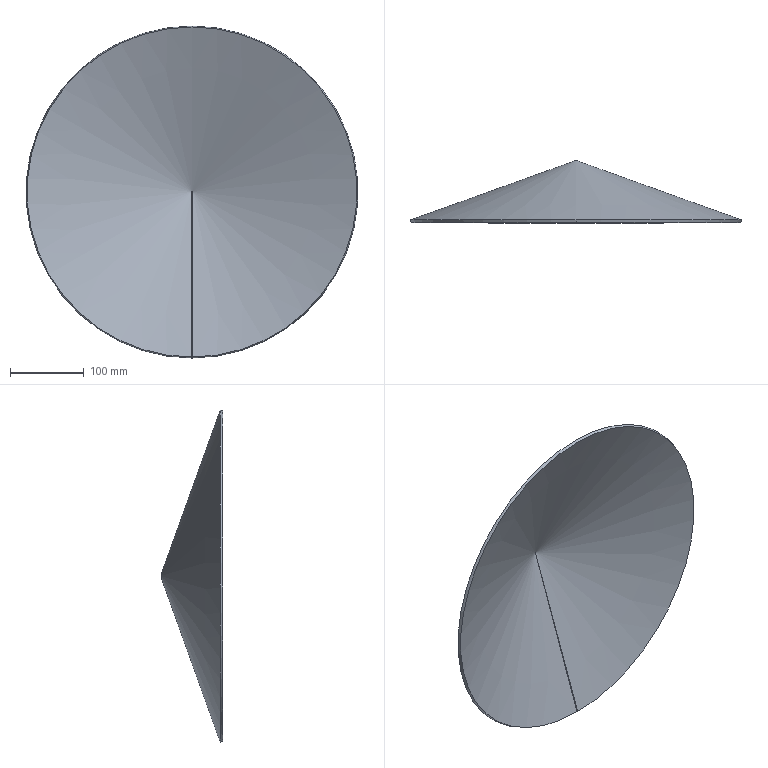Part | SolidWorks | features FlatPattern 1, LoftedBend 1, SheetMetal 1 | 1 solid | 8 faces | box 450 x 83.765 x 449.999 mm | volume 671050 mm3 | cone 6 | plane 2
STEP:
#1=CARTESIAN_POINT('',(0.,-3.765,223.649));
#2=VERTEX_POINT('',#1);
#3=CARTESIAN_POINT('',(-0.7807,-3.765,-223.648));
#4=VERTEX_POINT('',#3);
#5=CARTESIAN_POINT('',(0.,-3.765,0.));
#6=DIRECTION('',(0.,-1.,0.));
#7=DIRECTION('',(0.,0.,-1.));
#8=AXIS2_PLACEMENT_3D('',#5,#6,#7);
#9=CIRCLE('',#8,223.649);
#10=EDGE_CURVE('',#2,#4,#9,.T.);
#11=ORIENTED_EDGE('',*,*,#10,.F.);
#12=CARTESIAN_POINT('',(0.,0.,225.));
#13=VERTEX_POINT('',#12);
#14=CARTESIAN_POINT('',(0.,0.,225.));
#15=DIRECTION('',(0.,0.9413,0.3377));
#16=VECTOR('',#15,1000.);
#17=LINE('',#14,#16);
#18=EDGE_CURVE('',#2,#13,#17,.T.);
#19=ORIENTED_EDGE('',*,*,#18,.T.);
#20=CARTESIAN_POINT('',(-0.7854,0.,-224.999));
#21=VERTEX_POINT('',#20);
#22=CARTESIAN_POINT('',(0.,0.,0.));
#23=DIRECTION('',(0.,-1.,0.));
#24=DIRECTION('',(0.,0.,-1.));
#25=AXIS2_PLACEMENT_3D('',#22,#23,#24);
#26=CIRCLE('',#25,225.);
#27=EDGE_CURVE('',#13,#21,#26,.T.);
#28=ORIENTED_EDGE('',*,*,#27,.T.);
#29=CARTESIAN_POINT('',(-0.7854,0.,-224.999));
#30=DIRECTION('',(-0.001179,0.9413,-0.3377));
#31=VECTOR('',#30,1000.);
#32=LINE('',#29,#31);
#33=EDGE_CURVE('',#4,#21,#32,.T.);
#34=ORIENTED_EDGE('',*,*,#33,.F.);
#35=EDGE_LOOP('',(#11,#19,#28,#34));
#36=FACE_OUTER_BOUND('',#35,.T.);
#37=CARTESIAN_POINT('',(0.,0.,0.));
#38=DIRECTION('',(0.,1.,0.));
#39=DIRECTION('',(0.,0.,1.));
#40=AXIS2_PLACEMENT_3D('',#37,#38,#39);
#41=CONICAL_SURFACE('',#40,225.,0.3444);
#42=ADVANCED_FACE('',(#36),#41,.T.);
#43=CARTESIAN_POINT('',(0.002267,76.235,-0.6493));
#44=VERTEX_POINT('',#43);
#45=CARTESIAN_POINT('',(0.,76.235,0.6493));
#46=VERTEX_POINT('',#45);
#47=CARTESIAN_POINT('',(0.,76.235,0.));
#48=DIRECTION('',(0.,-1.,0.));
#49=DIRECTION('',(0.,0.,-1.));
#50=AXIS2_PLACEMENT_3D('',#47,#48,#49);
#51=CIRCLE('',#50,0.6493);
#52=EDGE_CURVE('',#44,#46,#51,.T.);
#53=ORIENTED_EDGE('',*,*,#52,.T.);
#54=CARTESIAN_POINT('',(0.,80.,2.));
#55=VERTEX_POINT('',#54);
#56=CARTESIAN_POINT('',(0.,80.,2.));
#57=DIRECTION('',(0.,0.9413,0.3377));
#58=VECTOR('',#57,1000.);
#59=LINE('',#56,#58);
#60=EDGE_CURVE('',#46,#55,#59,.T.);
#61=ORIENTED_EDGE('',*,*,#60,.T.);
#62=CARTESIAN_POINT('',(0.006981,80.,-2.));
#63=VERTEX_POINT('',#62);
#64=CARTESIAN_POINT('',(0.,80.,0.));
#65=DIRECTION('',(0.,-1.,0.));
#66=DIRECTION('',(0.,0.,-1.));
#67=AXIS2_PLACEMENT_3D('',#64,#65,#66);
#68=CIRCLE('',#67,2.);
#69=EDGE_CURVE('',#63,#55,#68,.T.);
#70=ORIENTED_EDGE('',*,*,#69,.F.);
#71=CARTESIAN_POINT('',(0.006981,80.,-2.));
#72=DIRECTION('',(0.001179,0.9413,-0.3377));
#73=VECTOR('',#72,1000.);
#74=LINE('',#71,#73);
#75=EDGE_CURVE('',#44,#63,#74,.T.);
#76=ORIENTED_EDGE('',*,*,#75,.F.);
#77=EDGE_LOOP('',(#53,#61,#70,#76));
#78=FACE_OUTER_BOUND('',#77,.T.);
#79=CARTESIAN_POINT('',(0.,80.,0.));
#80=DIRECTION('',(0.,1.,0.));
#81=DIRECTION('',(0.,0.,1.));
#82=AXIS2_PLACEMENT_3D('',#79,#80,#81);
#83=CONICAL_SURFACE('',#82,2.,0.3444);
#84=ADVANCED_FACE('',(#78),#83,.F.);
#85=CARTESIAN_POINT('',(0.7807,-3.765,-223.648));
#86=VERTEX_POINT('',#85);
#87=CARTESIAN_POINT('',(0.7854,0.,-224.999));
#88=VERTEX_POINT('',#87);
#89=CARTESIAN_POINT('',(0.7854,0.,-224.999));
#90=DIRECTION('',(0.001179,0.9413,-0.3377));
#91=VECTOR('',#90,1000.);
#92=LINE('',#89,#91);
#93=EDGE_CURVE('',#86,#88,#92,.T.);
#94=ORIENTED_EDGE('',*,*,#93,.F.);
#95=CARTESIAN_POINT('',(0.7807,-3.765,-223.648));
#96=DIRECTION('',(-0.003286,0.3377,0.9413));
#97=VECTOR('',#96,1000.);
#98=LINE('',#95,#97);
#99=EDGE_CURVE('',#86,#44,#98,.T.);
#100=ORIENTED_EDGE('',*,*,#99,.T.);
#101=ORIENTED_EDGE('',*,*,#75,.T.);
#102=CARTESIAN_POINT('',(0.7854,0.,-224.999));
#103=DIRECTION('',(-0.003286,0.3377,0.9413));
#104=VECTOR('',#103,1000.);
#105=LINE('',#102,#104);
#106=EDGE_CURVE('',#88,#63,#105,.T.);
#107=ORIENTED_EDGE('',*,*,#106,.F.);
#108=EDGE_LOOP('',(#94,#100,#101,#107));
#109=FACE_OUTER_BOUND('',#108,.T.);
#110=CARTESIAN_POINT('',(0.7854,0.,-224.999));
#111=DIRECTION('',(-1.,0.,-0.003491));
#112=DIRECTION('',(-0.003286,0.3377,0.9413));
#113=AXIS2_PLACEMENT_3D('',#110,#111,#112);
#114=PLANE('',#113);
#115=ADVANCED_FACE('',(#109),#114,.T.);
#116=ORIENTED_EDGE('',*,*,#60,.F.);
#117=CARTESIAN_POINT('',(-0.002267,76.235,-0.6493));
#118=VERTEX_POINT('',#117);
#119=CARTESIAN_POINT('',(0.,76.235,0.));
#120=DIRECTION('',(0.,-1.,0.));
#121=DIRECTION('',(0.,0.,-1.));
#122=AXIS2_PLACEMENT_3D('',#119,#120,#121);
#123=CIRCLE('',#122,0.6493);
#124=EDGE_CURVE('',#46,#118,#123,.T.);
#125=ORIENTED_EDGE('',*,*,#124,.T.);
#126=CARTESIAN_POINT('',(-0.006981,80.,-2.));
#127=VERTEX_POINT('',#126);
#128=CARTESIAN_POINT('',(-0.006981,80.,-2.));
#129=DIRECTION('',(-0.001179,0.9413,-0.3377));
#130=VECTOR('',#129,1000.);
#131=LINE('',#128,#130);
#132=EDGE_CURVE('',#118,#127,#131,.T.);
#133=ORIENTED_EDGE('',*,*,#132,.T.);
#134=CARTESIAN_POINT('',(0.,80.,0.));
#135=DIRECTION('',(0.,-1.,0.));
#136=DIRECTION('',(0.,0.,-1.));
#137=AXIS2_PLACEMENT_3D('',#134,#135,#136);
#138=CIRCLE('',#137,2.);
#139=EDGE_CURVE('',#55,#127,#138,.T.);
#140=ORIENTED_EDGE('',*,*,#139,.F.);
#141=EDGE_LOOP('',(#116,#125,#133,#140));
#142=FACE_OUTER_BOUND('',#141,.T.);
#143=CARTESIAN_POINT('',(0.,80.,0.));
#144=DIRECTION('',(0.,1.,0.));
#145=DIRECTION('',(0.,0.,1.));
#146=AXIS2_PLACEMENT_3D('',#143,#144,#145);
#147=CONICAL_SURFACE('',#146,2.,0.3444);
#148=ADVANCED_FACE('',(#142),#147,.F.);
#149=ORIENTED_EDGE('',*,*,#132,.F.);
#150=CARTESIAN_POINT('',(-0.7807,-3.765,-223.648));
#151=DIRECTION('',(0.003286,0.3377,0.9413));
#152=VECTOR('',#151,1000.);
#153=LINE('',#150,#152);
#154=EDGE_CURVE('',#4,#118,#153,.T.);
#155=ORIENTED_EDGE('',*,*,#154,.F.);
#156=ORIENTED_EDGE('',*,*,#33,.T.);
#157=CARTESIAN_POINT('',(-0.7854,0.,-224.999));
#158=DIRECTION('',(0.003286,0.3377,0.9413));
#159=VECTOR('',#158,1000.);
#160=LINE('',#157,#159);
#161=EDGE_CURVE('',#21,#127,#160,.T.);
#162=ORIENTED_EDGE('',*,*,#161,.T.);
#163=EDGE_LOOP('',(#149,#155,#156,#162));
#164=FACE_OUTER_BOUND('',#163,.T.);
#165=CARTESIAN_POINT('',(-0.7854,0.,-224.999));
#166=DIRECTION('',(-1.,0.,0.003491));
#167=DIRECTION('',(0.003286,0.3377,0.9413));
#168=AXIS2_PLACEMENT_3D('',#165,#166,#167);
#169=PLANE('',#168);
#170=ADVANCED_FACE('',(#164),#169,.F.);
#171=ORIENTED_EDGE('',*,*,#18,.F.);
#172=CARTESIAN_POINT('',(0.,-3.765,0.));
#173=DIRECTION('',(0.,-1.,0.));
#174=DIRECTION('',(0.,0.,-1.));
#175=AXIS2_PLACEMENT_3D('',#172,#173,#174);
#176=CIRCLE('',#175,223.649);
#177=EDGE_CURVE('',#86,#2,#176,.T.);
#178=ORIENTED_EDGE('',*,*,#177,.F.);
#179=ORIENTED_EDGE('',*,*,#93,.T.);
#180=CARTESIAN_POINT('',(0.,0.,0.));
#181=DIRECTION('',(0.,-1.,0.));
#182=DIRECTION('',(0.,0.,-1.));
#183=AXIS2_PLACEMENT_3D('',#180,#181,#182);
#184=CIRCLE('',#183,225.);
#185=EDGE_CURVE('',#88,#13,#184,.T.);
#186=ORIENTED_EDGE('',*,*,#185,.T.);
#187=EDGE_LOOP('',(#171,#178,#179,#186));
#188=FACE_OUTER_BOUND('',#187,.T.);
#189=CARTESIAN_POINT('',(0.,0.,0.));
#190=DIRECTION('',(0.,1.,0.));
#191=DIRECTION('',(0.,0.,1.));
#192=AXIS2_PLACEMENT_3D('',#189,#190,#191);
#193=CONICAL_SURFACE('',#192,225.,0.3444);
#194=ADVANCED_FACE('',(#188),#193,.T.);
#195=ORIENTED_EDGE('',*,*,#161,.F.);
#196=ORIENTED_EDGE('',*,*,#27,.F.);
#197=ORIENTED_EDGE('',*,*,#185,.F.);
#198=ORIENTED_EDGE('',*,*,#106,.T.);
#199=ORIENTED_EDGE('',*,*,#69,.T.);
#200=ORIENTED_EDGE('',*,*,#139,.T.);
#201=EDGE_LOOP('',(#195,#196,#197,#198,#199,#200));
#202=FACE_OUTER_BOUND('',#201,.T.);
#203=CARTESIAN_POINT('',(0.,0.,0.));
#204=DIRECTION('',(0.,-1.,0.));
#205=DIRECTION('',(0.,0.,-1.));
#206=AXIS2_PLACEMENT_3D('',#203,#204,#205);
#207=CONICAL_SURFACE('',#206,225.,1.226);
#208=ADVANCED_FACE('',(#202),#207,.T.);
#209=ORIENTED_EDGE('',*,*,#154,.T.);
#210=ORIENTED_EDGE('',*,*,#124,.F.);
#211=ORIENTED_EDGE('',*,*,#52,.F.);
#212=ORIENTED_EDGE('',*,*,#99,.F.);
#213=ORIENTED_EDGE('',*,*,#177,.T.);
#214=ORIENTED_EDGE('',*,*,#10,.T.);
#215=EDGE_LOOP('',(#209,#210,#211,#212,#213,#214));
#216=FACE_OUTER_BOUND('',#215,.T.);
#217=CARTESIAN_POINT('',(0.,-3.765,0.));
#218=DIRECTION('',(0.,-1.,0.));
#219=DIRECTION('',(0.,0.,-1.));
#220=AXIS2_PLACEMENT_3D('',#217,#218,#219);
#221=CONICAL_SURFACE('',#220,223.649,1.226);
#222=ADVANCED_FACE('',(#216),#221,.F.);
#223=CLOSED_SHELL('',(#42,#84,#115,#148,#170,#194,#208,#222));
#224=MANIFOLD_SOLID_BREP('',#223);
#225=CARTESIAN_POINT('',(0.,0.,0.));
#226=DIRECTION('',(0.,0.,1.));
#227=DIRECTION('',(1.,0.,0.));
#228=AXIS2_PLACEMENT_3D('',#225,#226,#227);
#229=(LENGTH_UNIT()NAMED_UNIT(*)SI_UNIT(.MILLI.,.METRE.));
#230=UNCERTAINTY_MEASURE_WITH_UNIT(LENGTH_MEASURE(0.00001),#229,'','');
#231=(NAMED_UNIT(*)PLANE_ANGLE_UNIT()SI_UNIT($,.RADIAN.));
#232=(NAMED_UNIT(*)SI_UNIT($,.STERADIAN.)SOLID_ANGLE_UNIT());
#233=(GEOMETRIC_REPRESENTATION_CONTEXT(3)GLOBAL_UNCERTAINTY_ASSIGNED_CONTEXT((#230))GLOBAL_UNIT_ASSIGNED_CONTEXT((#229,#231,#232))REPRESENTATION_CONTEXT('',''));
#234=ADVANCED_BREP_SHAPE_REPRESENTATION('',(#224,#228),#233);